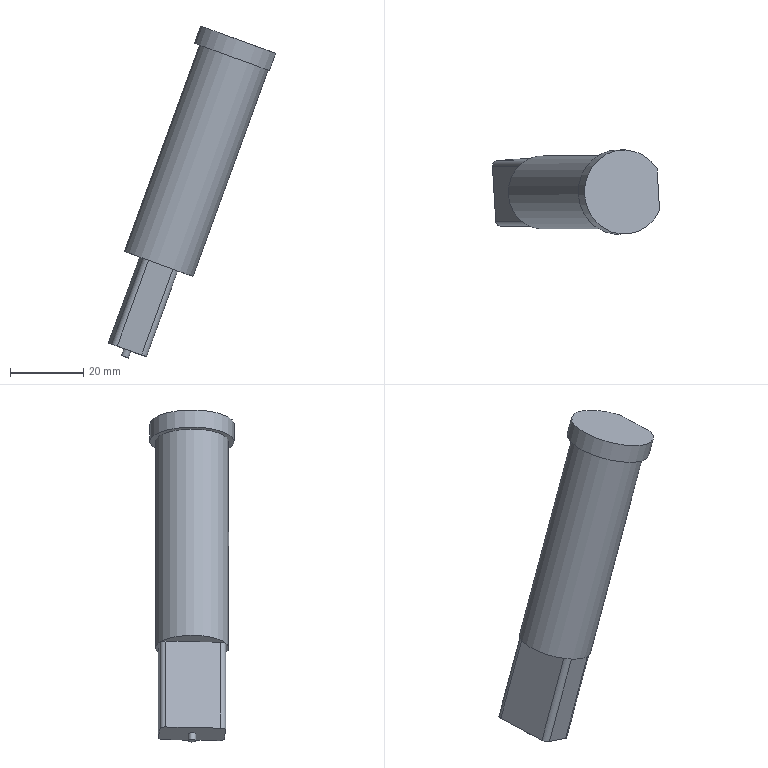Part | NX | features solid 2 | 1 solid | 17 faces | box 45.69 x 23 x 90.727 mm | volume 25372 mm3 | plane 10 | cylinder 7 | commonest cylinder face diameters 3 x4 2 x1 20 x1 23 x1
STEP:
#1=CARTESIAN_POINT('',(676.829,468.277,-16.259));
#2=VERTEX_POINT('',#1);
#3=CARTESIAN_POINT('',(686.207,468.917,-19.672));
#4=DIRECTION('',(-0.342,0.,-0.9397));
#5=DIRECTION('',(-0.9378,-0.06398,0.3413));
#6=AXIS2_PLACEMENT_3D('',#3,#4,#5);
#7=CIRCLE('',#6,10.);
#8=EDGE_CURVE('',#2,#2,#7,.T.);
#9=ORIENTED_EDGE('',*,*,#8,.T.);
#10=EDGE_LOOP('',(#9));
#11=FACE_BOUND('',#10,.T.);
#12=CARTESIAN_POINT('',(690.492,476.724,-21.231));
#13=VERTEX_POINT('',#12);
#14=CARTESIAN_POINT('',(691.394,461.755,-21.56));
#15=VERTEX_POINT('',#14);
#16=CARTESIAN_POINT('',(690.402,478.221,-21.199));
#17=DIRECTION('',(0.06013,-0.998,-0.02188));
#18=VECTOR('',#17,1000.);
#19=LINE('',#16,#18);
#20=EDGE_CURVE('',#13,#15,#19,.T.);
#21=ORIENTED_EDGE('',*,*,#20,.F.);
#22=CARTESIAN_POINT('',(688.995,478.125,-20.687));
#23=VERTEX_POINT('',#22);
#24=CARTESIAN_POINT('',(689.085,476.628,-20.719));
#25=DIRECTION('',(-0.342,0.,-0.9397));
#26=DIRECTION('',(-0.9378,-0.06398,0.3413));
#27=AXIS2_PLACEMENT_3D('',#24,#25,#26);
#28=CIRCLE('',#27,1.5);
#29=EDGE_CURVE('',#23,#13,#28,.T.);
#30=ORIENTED_EDGE('',*,*,#29,.F.);
#31=CARTESIAN_POINT('',(682.337,477.671,-18.263));
#32=VERTEX_POINT('',#31);
#33=CARTESIAN_POINT('',(680.93,477.575,-17.751));
#34=DIRECTION('',(0.9378,0.06398,-0.3413));
#35=VECTOR('',#34,1000.);
#36=LINE('',#33,#35);
#37=EDGE_CURVE('',#32,#23,#36,.T.);
#38=ORIENTED_EDGE('',*,*,#37,.F.);
#39=CARTESIAN_POINT('',(681.02,476.078,-17.784));
#40=VERTEX_POINT('',#39);
#41=CARTESIAN_POINT('',(682.427,476.174,-18.296));
#42=DIRECTION('',(-0.342,0.,-0.9397));
#43=DIRECTION('',(-0.9378,-0.06398,0.3413));
#44=AXIS2_PLACEMENT_3D('',#41,#42,#43);
#45=CIRCLE('',#44,1.5);
#46=EDGE_CURVE('',#40,#32,#45,.T.);
#47=ORIENTED_EDGE('',*,*,#46,.F.);
#48=CARTESIAN_POINT('',(681.922,461.109,-18.112));
#49=VERTEX_POINT('',#48);
#50=CARTESIAN_POINT('',(680.93,477.575,-17.751));
#51=DIRECTION('',(0.06013,-0.998,-0.02188));
#52=VECTOR('',#51,1000.);
#53=LINE('',#50,#52);
#54=EDGE_CURVE('',#40,#49,#53,.T.);
#55=ORIENTED_EDGE('',*,*,#54,.T.);
#56=CARTESIAN_POINT('',(683.419,459.708,-18.657));
#57=VERTEX_POINT('',#56);
#58=CARTESIAN_POINT('',(683.329,461.205,-18.624));
#59=DIRECTION('',(-0.342,0.,-0.9397));
#60=DIRECTION('',(-0.9378,-0.06398,0.3413));
#61=AXIS2_PLACEMENT_3D('',#58,#59,#60);
#62=CIRCLE('',#61,1.5);
#63=EDGE_CURVE('',#57,#49,#62,.T.);
#64=ORIENTED_EDGE('',*,*,#63,.F.);
#65=CARTESIAN_POINT('',(690.077,460.162,-21.081));
#66=VERTEX_POINT('',#65);
#67=CARTESIAN_POINT('',(691.484,460.258,-21.593));
#68=DIRECTION('',(-0.9378,-0.06398,0.3413));
#69=VECTOR('',#68,1000.);
#70=LINE('',#67,#69);
#71=EDGE_CURVE('',#66,#57,#70,.T.);
#72=ORIENTED_EDGE('',*,*,#71,.F.);
#73=CARTESIAN_POINT('',(689.987,461.659,-21.048));
#74=DIRECTION('',(-0.342,0.,-0.9397));
#75=DIRECTION('',(-0.9378,-0.06398,0.3413));
#76=AXIS2_PLACEMENT_3D('',#73,#74,#75);
#77=CIRCLE('',#76,1.5);
#78=EDGE_CURVE('',#15,#66,#77,.T.);
#79=ORIENTED_EDGE('',*,*,#78,.F.);
#80=EDGE_LOOP('',(#21,#30,#38,#47,#55,#64,#72,#79));
#81=FACE_BOUND('',#80,.T.);
#82=CARTESIAN_POINT('',(686.207,468.917,-19.672));
#83=DIRECTION('',(0.342,0.,0.9397));
#84=DIRECTION('',(-0.9378,-0.06398,0.3413));
#85=AXIS2_PLACEMENT_3D('',#82,#83,#84);
#86=PLANE('',#85);
#87=ADVANCED_FACE('',(#11,#81),#86,.F.);
#88=ORIENTED_EDGE('',*,*,#8,.F.);
#89=EDGE_LOOP('',(#88));
#90=FACE_BOUND('',#89,.T.);
#91=CARTESIAN_POINT('',(716.106,469.556,33.296));
#92=VERTEX_POINT('',#91);
#93=CARTESIAN_POINT('',(706.728,468.917,36.71));
#94=DIRECTION('',(-0.342,0.,-0.9397));
#95=DIRECTION('',(-0.9378,-0.06398,0.3413));
#96=AXIS2_PLACEMENT_3D('',#93,#94,#95);
#97=CIRCLE('',#96,10.);
#98=EDGE_CURVE('',#92,#92,#97,.T.);
#99=ORIENTED_EDGE('',*,*,#98,.T.);
#100=EDGE_LOOP('',(#99));
#101=FACE_BOUND('',#100,.T.);
#102=CARTESIAN_POINT('',(708.438,468.917,41.408));
#103=DIRECTION('',(-0.342,0.,-0.9397));
#104=DIRECTION('',(0.9378,0.06398,-0.3413));
#105=AXIS2_PLACEMENT_3D('',#102,#103,#104);
#106=CYLINDRICAL_SURFACE('',#105,10.);
#107=ADVANCED_FACE('',(#90,#101),#106,.T.);
#108=CARTESIAN_POINT('',(716.447,463.889,33.172));
#109=VERTEX_POINT('',#108);
#110=CARTESIAN_POINT('',(715.764,475.224,33.421));
#111=VERTEX_POINT('',#110);
#112=CARTESIAN_POINT('',(706.728,468.917,36.71));
#113=DIRECTION('',(-0.342,0.,-0.9397));
#114=DIRECTION('',(-0.9378,-0.06398,0.3413));
#115=AXIS2_PLACEMENT_3D('',#112,#113,#114);
#116=CIRCLE('',#115,11.5);
#117=EDGE_CURVE('',#109,#111,#116,.T.);
#118=ORIENTED_EDGE('',*,*,#117,.T.);
#119=CARTESIAN_POINT('',(716.106,469.556,33.296));
#120=DIRECTION('',(-0.06013,0.998,0.02188));
#121=VECTOR('',#120,1000.);
#122=LINE('',#119,#121);
#123=EDGE_CURVE('',#92,#111,#122,.T.);
#124=ORIENTED_EDGE('',*,*,#123,.F.);
#125=ORIENTED_EDGE('',*,*,#98,.F.);
#126=CARTESIAN_POINT('',(716.106,469.556,33.296));
#127=DIRECTION('',(-0.06013,0.998,0.02188));
#128=VECTOR('',#127,1000.);
#129=LINE('',#126,#128);
#130=EDGE_CURVE('',#109,#92,#129,.T.);
#131=ORIENTED_EDGE('',*,*,#130,.F.);
#132=EDGE_LOOP('',(#118,#124,#125,#131));
#133=FACE_BOUND('',#132,.T.);
#134=CARTESIAN_POINT('',(706.728,468.917,36.71));
#135=DIRECTION('',(0.342,0.,0.9397));
#136=DIRECTION('',(-0.9378,-0.06398,0.3413));
#137=AXIS2_PLACEMENT_3D('',#134,#135,#136);
#138=PLANE('',#137);
#139=ADVANCED_FACE('',(#133),#138,.F.);
#140=CARTESIAN_POINT('',(717.474,475.224,38.119));
#141=VERTEX_POINT('',#140);
#142=CARTESIAN_POINT('',(718.843,475.224,41.878));
#143=DIRECTION('',(-0.342,0.,-0.9397));
#144=VECTOR('',#143,1000.);
#145=LINE('',#142,#144);
#146=EDGE_CURVE('',#141,#111,#145,.T.);
#147=ORIENTED_EDGE('',*,*,#146,.T.);
#148=ORIENTED_EDGE('',*,*,#117,.F.);
#149=CARTESIAN_POINT('',(718.157,463.889,37.871));
#150=VERTEX_POINT('',#149);
#151=CARTESIAN_POINT('',(719.525,463.889,41.629));
#152=DIRECTION('',(-0.342,0.,-0.9397));
#153=VECTOR('',#152,1000.);
#154=LINE('',#151,#153);
#155=EDGE_CURVE('',#109,#150,#154,.F.);
#156=ORIENTED_EDGE('',*,*,#155,.T.);
#157=CARTESIAN_POINT('',(708.438,468.917,41.408));
#158=DIRECTION('',(-0.342,0.,-0.9397));
#159=DIRECTION('',(-0.9378,-0.06398,0.3413));
#160=AXIS2_PLACEMENT_3D('',#157,#158,#159);
#161=CIRCLE('',#160,11.5);
#162=EDGE_CURVE('',#150,#141,#161,.T.);
#163=ORIENTED_EDGE('',*,*,#162,.T.);
#164=EDGE_LOOP('',(#147,#148,#156,#163));
#165=FACE_BOUND('',#164,.T.);
#166=CARTESIAN_POINT('',(706.728,468.917,36.71));
#167=DIRECTION('',(0.342,0.,0.9397));
#168=DIRECTION('',(-0.9378,-0.06398,0.3413));
#169=AXIS2_PLACEMENT_3D('',#166,#167,#168);
#170=CYLINDRICAL_SURFACE('',#169,11.5);
#171=ADVANCED_FACE('',(#165),#170,.T.);
#172=CARTESIAN_POINT('',(717.816,469.556,37.995));
#173=DIRECTION('',(-0.06013,0.998,0.02188));
#174=VECTOR('',#173,1000.);
#175=LINE('',#172,#174);
#176=EDGE_CURVE('',#150,#141,#175,.T.);
#177=ORIENTED_EDGE('',*,*,#176,.T.);
#178=ORIENTED_EDGE('',*,*,#162,.F.);
#179=EDGE_LOOP('',(#177,#178));
#180=FACE_BOUND('',#179,.T.);
#181=CARTESIAN_POINT('',(708.438,468.917,41.408));
#182=DIRECTION('',(0.342,0.,0.9397));
#183=DIRECTION('',(-0.9378,-0.06398,0.3413));
#184=AXIS2_PLACEMENT_3D('',#181,#182,#183);
#185=PLANE('',#184);
#186=ADVANCED_FACE('',(#180),#185,.T.);
#187=ORIENTED_EDGE('',*,*,#155,.F.);
#188=ORIENTED_EDGE('',*,*,#130,.T.);
#189=ORIENTED_EDGE('',*,*,#123,.T.);
#190=ORIENTED_EDGE('',*,*,#146,.F.);
#191=ORIENTED_EDGE('',*,*,#176,.F.);
#192=EDGE_LOOP('',(#187,#188,#189,#190,#191));
#193=FACE_BOUND('',#192,.T.);
#194=CARTESIAN_POINT('',(718.843,475.224,41.878));
#195=DIRECTION('',(-0.9378,-0.06398,0.3413));
#196=DIRECTION('',(-0.342,0.,-0.9397));
#197=AXIS2_PLACEMENT_3D('',#194,#195,#196);
#198=PLANE('',#197);
#199=ADVANCED_FACE('',(#193),#198,.F.);
#200=CARTESIAN_POINT('',(681.527,460.162,-44.573));
#201=VERTEX_POINT('',#200);
#202=CARTESIAN_POINT('',(674.868,459.708,-42.15));
#203=VERTEX_POINT('',#202);
#204=CARTESIAN_POINT('',(682.933,460.258,-45.085));
#205=DIRECTION('',(-0.9378,-0.06398,0.3413));
#206=VECTOR('',#205,1000.);
#207=LINE('',#204,#206);
#208=EDGE_CURVE('',#201,#203,#207,.T.);
#209=ORIENTED_EDGE('',*,*,#208,.F.);
#210=CARTESIAN_POINT('',(681.527,460.162,-44.573));
#211=DIRECTION('',(0.342,0.,0.9397));
#212=VECTOR('',#211,1000.);
#213=LINE('',#210,#212);
#214=EDGE_CURVE('',#66,#201,#213,.F.);
#215=ORIENTED_EDGE('',*,*,#214,.F.);
#216=ORIENTED_EDGE('',*,*,#71,.T.);
#217=CARTESIAN_POINT('',(683.419,459.708,-18.657));
#218=DIRECTION('',(0.342,0.,0.9397));
#219=VECTOR('',#218,1000.);
#220=LINE('',#217,#219);
#221=EDGE_CURVE('',#203,#57,#220,.T.);
#222=ORIENTED_EDGE('',*,*,#221,.F.);
#223=EDGE_LOOP('',(#209,#215,#216,#222));
#224=FACE_BOUND('',#223,.T.);
#225=CARTESIAN_POINT('',(682.933,460.258,-45.085));
#226=DIRECTION('',(0.06013,-0.998,-0.02188));
#227=DIRECTION('',(-0.342,0.,-0.9397));
#228=AXIS2_PLACEMENT_3D('',#225,#226,#227);
#229=PLANE('',#228);
#230=ADVANCED_FACE('',(#224),#229,.T.);
#231=CARTESIAN_POINT('',(672.47,476.078,-41.276));
#232=VERTEX_POINT('',#231);
#233=CARTESIAN_POINT('',(673.372,461.109,-41.605));
#234=VERTEX_POINT('',#233);
#235=CARTESIAN_POINT('',(672.38,477.575,-41.244));
#236=DIRECTION('',(0.06013,-0.998,-0.02188));
#237=VECTOR('',#236,1000.);
#238=LINE('',#235,#237);
#239=EDGE_CURVE('',#232,#234,#238,.T.);
#240=ORIENTED_EDGE('',*,*,#239,.T.);
#241=CARTESIAN_POINT('',(673.372,461.109,-41.605));
#242=DIRECTION('',(0.342,0.,0.9397));
#243=VECTOR('',#242,1000.);
#244=LINE('',#241,#243);
#245=EDGE_CURVE('',#49,#234,#244,.F.);
#246=ORIENTED_EDGE('',*,*,#245,.F.);
#247=ORIENTED_EDGE('',*,*,#54,.F.);
#248=CARTESIAN_POINT('',(681.02,476.078,-17.784));
#249=DIRECTION('',(0.342,0.,0.9397));
#250=VECTOR('',#249,1000.);
#251=LINE('',#248,#250);
#252=EDGE_CURVE('',#232,#40,#251,.T.);
#253=ORIENTED_EDGE('',*,*,#252,.F.);
#254=EDGE_LOOP('',(#240,#246,#247,#253));
#255=FACE_BOUND('',#254,.T.);
#256=CARTESIAN_POINT('',(672.38,477.575,-41.244));
#257=DIRECTION('',(0.9378,0.06398,-0.3413));
#258=DIRECTION('',(0.342,0.,0.9397));
#259=AXIS2_PLACEMENT_3D('',#256,#257,#258);
#260=PLANE('',#259);
#261=ADVANCED_FACE('',(#255),#260,.F.);
#262=ORIENTED_EDGE('',*,*,#37,.T.);
#263=CARTESIAN_POINT('',(680.444,478.125,-44.179));
#264=VERTEX_POINT('',#263);
#265=CARTESIAN_POINT('',(680.444,478.125,-44.179));
#266=DIRECTION('',(0.342,0.,0.9397));
#267=VECTOR('',#266,1000.);
#268=LINE('',#265,#267);
#269=EDGE_CURVE('',#264,#23,#268,.T.);
#270=ORIENTED_EDGE('',*,*,#269,.F.);
#271=CARTESIAN_POINT('',(673.786,477.671,-41.756));
#272=VERTEX_POINT('',#271);
#273=CARTESIAN_POINT('',(672.38,477.575,-41.244));
#274=DIRECTION('',(0.9378,0.06398,-0.3413));
#275=VECTOR('',#274,1000.);
#276=LINE('',#273,#275);
#277=EDGE_CURVE('',#272,#264,#276,.T.);
#278=ORIENTED_EDGE('',*,*,#277,.F.);
#279=CARTESIAN_POINT('',(673.786,477.671,-41.756));
#280=DIRECTION('',(0.342,0.,0.9397));
#281=VECTOR('',#280,1000.);
#282=LINE('',#279,#281);
#283=EDGE_CURVE('',#32,#272,#282,.F.);
#284=ORIENTED_EDGE('',*,*,#283,.F.);
#285=EDGE_LOOP('',(#262,#270,#278,#284));
#286=FACE_BOUND('',#285,.T.);
#287=CARTESIAN_POINT('',(672.38,477.575,-41.244));
#288=DIRECTION('',(-0.06013,0.998,0.02188));
#289=DIRECTION('',(0.342,0.,0.9397));
#290=AXIS2_PLACEMENT_3D('',#287,#288,#289);
#291=PLANE('',#290);
#292=ADVANCED_FACE('',(#286),#291,.T.);
#293=ORIENTED_EDGE('',*,*,#20,.T.);
#294=CARTESIAN_POINT('',(682.843,461.755,-45.052));
#295=VERTEX_POINT('',#294);
#296=CARTESIAN_POINT('',(682.843,461.755,-45.052));
#297=DIRECTION('',(0.342,0.,0.9397));
#298=VECTOR('',#297,1000.);
#299=LINE('',#296,#298);
#300=EDGE_CURVE('',#295,#15,#299,.T.);
#301=ORIENTED_EDGE('',*,*,#300,.F.);
#302=CARTESIAN_POINT('',(681.941,476.724,-44.724));
#303=VERTEX_POINT('',#302);
#304=CARTESIAN_POINT('',(681.851,478.221,-44.691));
#305=DIRECTION('',(0.06013,-0.998,-0.02188));
#306=VECTOR('',#305,1000.);
#307=LINE('',#304,#306);
#308=EDGE_CURVE('',#303,#295,#307,.T.);
#309=ORIENTED_EDGE('',*,*,#308,.F.);
#310=CARTESIAN_POINT('',(681.941,476.724,-44.724));
#311=DIRECTION('',(0.342,0.,0.9397));
#312=VECTOR('',#311,1000.);
#313=LINE('',#310,#312);
#314=EDGE_CURVE('',#13,#303,#313,.F.);
#315=ORIENTED_EDGE('',*,*,#314,.F.);
#316=EDGE_LOOP('',(#293,#301,#309,#315));
#317=FACE_BOUND('',#316,.T.);
#318=CARTESIAN_POINT('',(681.851,478.221,-44.691));
#319=DIRECTION('',(0.9378,0.06398,-0.3413));
#320=DIRECTION('',(0.342,0.,0.9397));
#321=AXIS2_PLACEMENT_3D('',#318,#319,#320);
#322=PLANE('',#321);
#323=ADVANCED_FACE('',(#317),#322,.T.);
#324=CARTESIAN_POINT('',(678.594,468.981,-43.506));
#325=VERTEX_POINT('',#324);
#326=CARTESIAN_POINT('',(677.656,468.917,-43.164));
#327=DIRECTION('',(0.342,0.,0.9397));
#328=DIRECTION('',(0.9378,0.06398,-0.3413));
#329=AXIS2_PLACEMENT_3D('',#326,#327,#328);
#330=CIRCLE('',#329,1.);
#331=EDGE_CURVE('',#325,#325,#330,.T.);
#332=ORIENTED_EDGE('',*,*,#331,.T.);
#333=EDGE_LOOP('',(#332));
#334=FACE_BOUND('',#333,.T.);
#335=ORIENTED_EDGE('',*,*,#277,.T.);
#336=CARTESIAN_POINT('',(680.535,476.628,-44.212));
#337=DIRECTION('',(0.342,0.,0.9397));
#338=DIRECTION('',(0.9378,0.06398,-0.3413));
#339=AXIS2_PLACEMENT_3D('',#336,#337,#338);
#340=CIRCLE('',#339,1.5);
#341=EDGE_CURVE('',#303,#264,#340,.T.);
#342=ORIENTED_EDGE('',*,*,#341,.F.);
#343=ORIENTED_EDGE('',*,*,#308,.T.);
#344=CARTESIAN_POINT('',(681.436,461.659,-44.54));
#345=DIRECTION('',(0.342,0.,0.9397));
#346=DIRECTION('',(0.9378,0.06398,-0.3413));
#347=AXIS2_PLACEMENT_3D('',#344,#345,#346);
#348=CIRCLE('',#347,1.5);
#349=EDGE_CURVE('',#201,#295,#348,.T.);
#350=ORIENTED_EDGE('',*,*,#349,.F.);
#351=ORIENTED_EDGE('',*,*,#208,.T.);
#352=CARTESIAN_POINT('',(674.778,461.205,-42.117));
#353=DIRECTION('',(0.342,0.,0.9397));
#354=DIRECTION('',(0.9378,0.06398,-0.3413));
#355=AXIS2_PLACEMENT_3D('',#352,#353,#354);
#356=CIRCLE('',#355,1.5);
#357=EDGE_CURVE('',#234,#203,#356,.T.);
#358=ORIENTED_EDGE('',*,*,#357,.F.);
#359=ORIENTED_EDGE('',*,*,#239,.F.);
#360=CARTESIAN_POINT('',(673.876,476.174,-41.788));
#361=DIRECTION('',(0.342,0.,0.9397));
#362=DIRECTION('',(0.9378,0.06398,-0.3413));
#363=AXIS2_PLACEMENT_3D('',#360,#361,#362);
#364=CIRCLE('',#363,1.5);
#365=EDGE_CURVE('',#272,#232,#364,.T.);
#366=ORIENTED_EDGE('',*,*,#365,.F.);
#367=EDGE_LOOP('',(#335,#342,#343,#350,#351,#358,#359,#366));
#368=FACE_BOUND('',#367,.T.);
#369=CARTESIAN_POINT('',(673.462,459.612,-41.638));
#370=DIRECTION('',(-0.342,0.,-0.9397));
#371=DIRECTION('',(0.9378,0.06398,-0.3413));
#372=AXIS2_PLACEMENT_3D('',#369,#370,#371);
#373=PLANE('',#372);
#374=ADVANCED_FACE('',(#334,#368),#373,.T.);
#375=ORIENTED_EDGE('',*,*,#365,.T.);
#376=ORIENTED_EDGE('',*,*,#252,.T.);
#377=ORIENTED_EDGE('',*,*,#46,.T.);
#378=ORIENTED_EDGE('',*,*,#283,.T.);
#379=EDGE_LOOP('',(#375,#376,#377,#378));
#380=FACE_BOUND('',#379,.T.);
#381=CARTESIAN_POINT('',(673.876,476.174,-41.788));
#382=DIRECTION('',(-0.342,0.,-0.9397));
#383=DIRECTION('',(0.9378,0.06398,-0.3413));
#384=AXIS2_PLACEMENT_3D('',#381,#382,#383);
#385=CYLINDRICAL_SURFACE('',#384,1.5);
#386=ADVANCED_FACE('',(#380),#385,.T.);
#387=ORIENTED_EDGE('',*,*,#341,.T.);
#388=ORIENTED_EDGE('',*,*,#269,.T.);
#389=ORIENTED_EDGE('',*,*,#29,.T.);
#390=ORIENTED_EDGE('',*,*,#314,.T.);
#391=EDGE_LOOP('',(#387,#388,#389,#390));
#392=FACE_BOUND('',#391,.T.);
#393=CARTESIAN_POINT('',(680.535,476.628,-44.212));
#394=DIRECTION('',(0.342,0.,0.9397));
#395=DIRECTION('',(-0.9378,-0.06398,0.3413));
#396=AXIS2_PLACEMENT_3D('',#393,#394,#395);
#397=CYLINDRICAL_SURFACE('',#396,1.5);
#398=ADVANCED_FACE('',(#392),#397,.T.);
#399=ORIENTED_EDGE('',*,*,#357,.T.);
#400=ORIENTED_EDGE('',*,*,#221,.T.);
#401=ORIENTED_EDGE('',*,*,#63,.T.);
#402=ORIENTED_EDGE('',*,*,#245,.T.);
#403=EDGE_LOOP('',(#399,#400,#401,#402));
#404=FACE_BOUND('',#403,.T.);
#405=CARTESIAN_POINT('',(674.778,461.205,-42.117));
#406=DIRECTION('',(-0.342,0.,-0.9397));
#407=DIRECTION('',(0.9378,0.06398,-0.3413));
#408=AXIS2_PLACEMENT_3D('',#405,#406,#407);
#409=CYLINDRICAL_SURFACE('',#408,1.5);
#410=ADVANCED_FACE('',(#404),#409,.T.);
#411=ORIENTED_EDGE('',*,*,#349,.T.);
#412=ORIENTED_EDGE('',*,*,#300,.T.);
#413=ORIENTED_EDGE('',*,*,#78,.T.);
#414=ORIENTED_EDGE('',*,*,#214,.T.);
#415=EDGE_LOOP('',(#411,#412,#413,#414));
#416=FACE_BOUND('',#415,.T.);
#417=CARTESIAN_POINT('',(681.436,461.659,-44.54));
#418=DIRECTION('',(0.342,0.,0.9397));
#419=DIRECTION('',(-0.9378,-0.06398,0.3413));
#420=AXIS2_PLACEMENT_3D('',#417,#418,#419);
#421=CYLINDRICAL_SURFACE('',#420,1.5);
#422=ADVANCED_FACE('',(#416),#421,.T.);
#423=CARTESIAN_POINT('',(676.035,468.853,-44.702));
#424=VERTEX_POINT('',#423);
#425=CARTESIAN_POINT('',(676.972,468.917,-45.044));
#426=DIRECTION('',(-0.342,0.,-0.9397));
#427=DIRECTION('',(-0.9378,-0.06398,0.3413));
#428=AXIS2_PLACEMENT_3D('',#425,#426,#427);
#429=CIRCLE('',#428,1.);
#430=EDGE_CURVE('',#424,#424,#429,.T.);
#431=ORIENTED_EDGE('',*,*,#430,.F.);
#432=EDGE_LOOP('',(#431));
#433=FACE_BOUND('',#432,.T.);
#434=ORIENTED_EDGE('',*,*,#331,.F.);
#435=EDGE_LOOP('',(#434));
#436=FACE_BOUND('',#435,.T.);
#437=CARTESIAN_POINT('',(676.972,468.917,-45.044));
#438=DIRECTION('',(0.342,0.,0.9397));
#439=DIRECTION('',(-0.9378,-0.06398,0.3413));
#440=AXIS2_PLACEMENT_3D('',#437,#438,#439);
#441=CYLINDRICAL_SURFACE('',#440,1.);
#442=ADVANCED_FACE('',(#433,#436),#441,.T.);
#443=ORIENTED_EDGE('',*,*,#430,.T.);
#444=EDGE_LOOP('',(#443));
#445=FACE_BOUND('',#444,.T.);
#446=CARTESIAN_POINT('',(676.972,468.917,-45.044));
#447=DIRECTION('',(0.342,0.,0.9397));
#448=DIRECTION('',(-0.9378,-0.06398,0.3413));
#449=AXIS2_PLACEMENT_3D('',#446,#447,#448);
#450=PLANE('',#449);
#451=ADVANCED_FACE('',(#445),#450,.F.);
#452=CLOSED_SHELL('',(#87,#107,#139,#171,#186,#199,#230,#261,#292,#323,#374,#386,#398,#410,#422,#442,#451));
#453=MANIFOLD_SOLID_BREP('',#452);
#454=(LENGTH_UNIT()NAMED_UNIT(*)SI_UNIT(.MILLI.,.METRE.));
#455=UNCERTAINTY_MEASURE_WITH_UNIT(LENGTH_MEASURE(0.00001),#454,'','');
#456=(NAMED_UNIT(*)PLANE_ANGLE_UNIT()SI_UNIT($,.RADIAN.));
#457=(NAMED_UNIT(*)SI_UNIT($,.STERADIAN.)SOLID_ANGLE_UNIT());
#458=(GEOMETRIC_REPRESENTATION_CONTEXT(3)GLOBAL_UNCERTAINTY_ASSIGNED_CONTEXT((#455))GLOBAL_UNIT_ASSIGNED_CONTEXT((#454,#456,#457))REPRESENTATION_CONTEXT('',''));
#459=ADVANCED_BREP_SHAPE_REPRESENTATION('',(#453),#458);